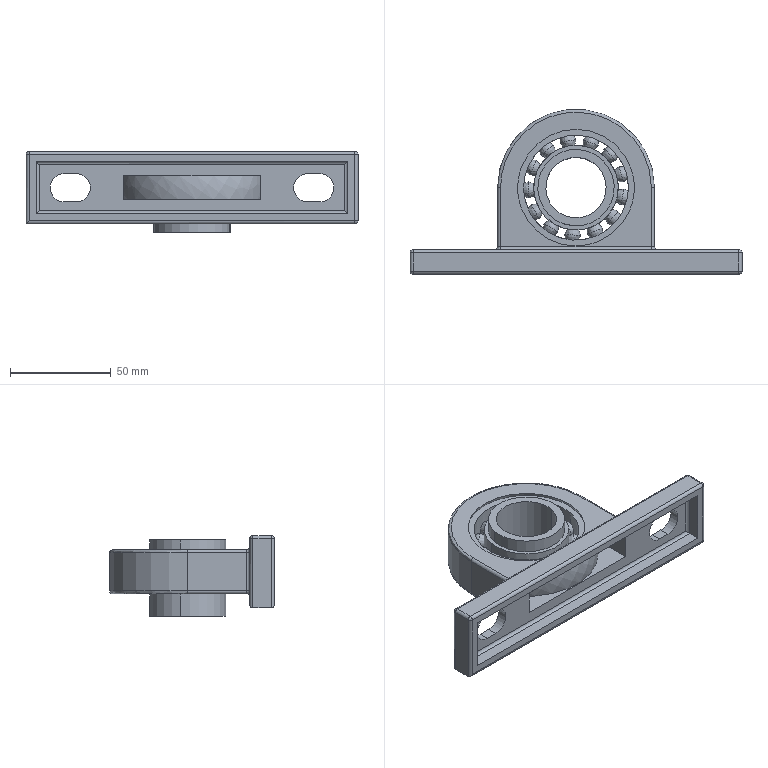Part | SolidWorks | features LayoutProfileFeature 1 | 2 solids | 110 faces | volume 115965 mm3 | spline 43 | cylinder 38 | plane 29 | commonest cylinder face diameters 3 x23 14 x4 38 x4 30 x2 42.044 x2 52.213 x2